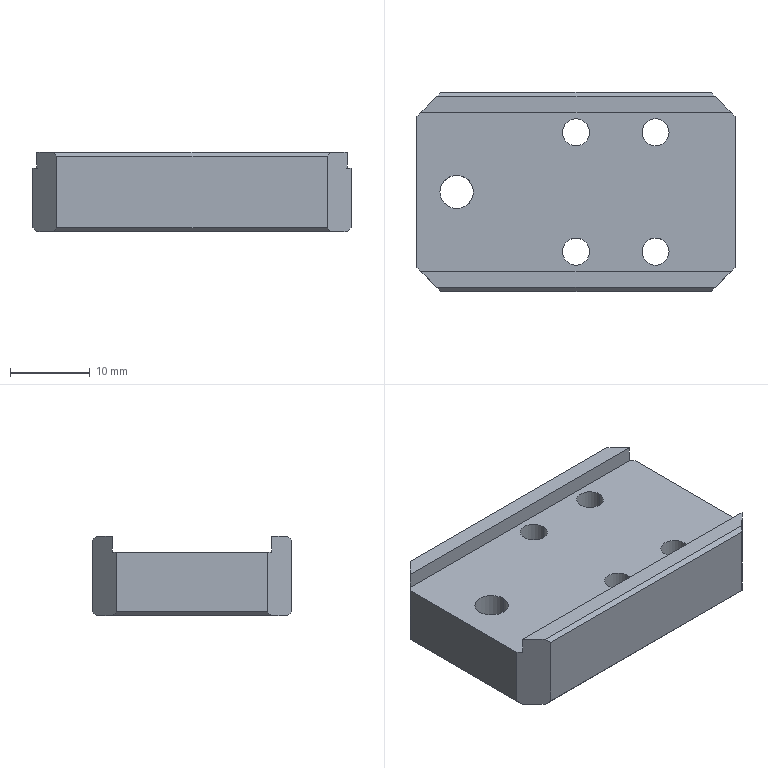Part | SolidWorks | features Chamfer 2, HoleWzd 2, Extrusion 1, ICE 1 | 1 solid | 42 faces | box 40 x 25 x 10 mm | volume 7537 mm3 | plane 24 | cylinder 18 | commonest cylinder face diameters 3.4 x8 6 x8 4.2 x2
STEP:
#1=CARTESIAN_POINT('',(13.,7.5,3.4));
#2=VERTEX_POINT('',#1);
#3=CARTESIAN_POINT('',(7.,7.5,3.4));
#4=VERTEX_POINT('',#3);
#5=CARTESIAN_POINT('',(10.,7.5,3.4));
#6=DIRECTION('',(0.,0.,-1.));
#7=DIRECTION('',(-1.,0.,0.));
#8=AXIS2_PLACEMENT_3D('',#5,#6,#7);
#9=CIRCLE('',#8,3.);
#10=EDGE_CURVE('',#2,#4,#9,.T.);
#11=ORIENTED_EDGE('',*,*,#10,.F.);
#12=CARTESIAN_POINT('',(13.,7.5,0.));
#13=VERTEX_POINT('',#12);
#14=CARTESIAN_POINT('',(13.,7.5,0.));
#15=DIRECTION('',(0.,0.,-1.));
#16=VECTOR('',#15,1000.);
#17=LINE('',#14,#16);
#18=EDGE_CURVE('',#2,#13,#17,.T.);
#19=ORIENTED_EDGE('',*,*,#18,.T.);
#20=CARTESIAN_POINT('',(7.,7.5,0.));
#21=VERTEX_POINT('',#20);
#22=CARTESIAN_POINT('',(10.,7.5,0.));
#23=DIRECTION('',(0.,0.,-1.));
#24=DIRECTION('',(-1.,0.,0.));
#25=AXIS2_PLACEMENT_3D('',#22,#23,#24);
#26=CIRCLE('',#25,3.);
#27=EDGE_CURVE('',#13,#21,#26,.T.);
#28=ORIENTED_EDGE('',*,*,#27,.T.);
#29=CARTESIAN_POINT('',(7.,7.5,0.));
#30=DIRECTION('',(0.,0.,-1.));
#31=VECTOR('',#30,1000.);
#32=LINE('',#29,#31);
#33=EDGE_CURVE('',#4,#21,#32,.T.);
#34=ORIENTED_EDGE('',*,*,#33,.F.);
#35=EDGE_LOOP('',(#11,#19,#28,#34));
#36=FACE_OUTER_BOUND('',#35,.T.);
#37=CARTESIAN_POINT('',(10.,7.5,0.));
#38=DIRECTION('',(0.,0.,-1.));
#39=DIRECTION('',(-1.,0.,0.));
#40=AXIS2_PLACEMENT_3D('',#37,#38,#39);
#41=CYLINDRICAL_SURFACE('',#40,3.);
#42=ADVANCED_FACE('',(#36),#41,.F.);
#43=CARTESIAN_POINT('',(11.7,7.5,8.));
#44=VERTEX_POINT('',#43);
#45=CARTESIAN_POINT('',(8.3,7.5,8.));
#46=VERTEX_POINT('',#45);
#47=CARTESIAN_POINT('',(10.,7.5,8.));
#48=DIRECTION('',(0.,0.,-1.));
#49=DIRECTION('',(-1.,0.,0.));
#50=AXIS2_PLACEMENT_3D('',#47,#48,#49);
#51=CIRCLE('',#50,1.7);
#52=EDGE_CURVE('',#44,#46,#51,.T.);
#53=ORIENTED_EDGE('',*,*,#52,.F.);
#54=CARTESIAN_POINT('',(11.7,7.5,3.4));
#55=VERTEX_POINT('',#54);
#56=CARTESIAN_POINT('',(11.7,7.5,0.));
#57=DIRECTION('',(0.,0.,-1.));
#58=VECTOR('',#57,1000.);
#59=LINE('',#56,#58);
#60=EDGE_CURVE('',#44,#55,#59,.T.);
#61=ORIENTED_EDGE('',*,*,#60,.T.);
#62=CARTESIAN_POINT('',(8.3,7.5,3.4));
#63=VERTEX_POINT('',#62);
#64=CARTESIAN_POINT('',(10.,7.5,3.4));
#65=DIRECTION('',(0.,0.,-1.));
#66=DIRECTION('',(-1.,0.,0.));
#67=AXIS2_PLACEMENT_3D('',#64,#65,#66);
#68=CIRCLE('',#67,1.7);
#69=EDGE_CURVE('',#55,#63,#68,.T.);
#70=ORIENTED_EDGE('',*,*,#69,.T.);
#71=CARTESIAN_POINT('',(8.3,7.5,0.));
#72=DIRECTION('',(0.,0.,-1.));
#73=VECTOR('',#72,1000.);
#74=LINE('',#71,#73);
#75=EDGE_CURVE('',#46,#63,#74,.T.);
#76=ORIENTED_EDGE('',*,*,#75,.F.);
#77=EDGE_LOOP('',(#53,#61,#70,#76));
#78=FACE_OUTER_BOUND('',#77,.T.);
#79=CARTESIAN_POINT('',(10.,7.5,0.));
#80=DIRECTION('',(0.,0.,-1.));
#81=DIRECTION('',(-1.,0.,0.));
#82=AXIS2_PLACEMENT_3D('',#79,#80,#81);
#83=CYLINDRICAL_SURFACE('',#82,1.7);
#84=ADVANCED_FACE('',(#78),#83,.F.);
#85=CARTESIAN_POINT('',(13.,-7.5,3.4));
#86=VERTEX_POINT('',#85);
#87=CARTESIAN_POINT('',(7.,-7.5,3.4));
#88=VERTEX_POINT('',#87);
#89=CARTESIAN_POINT('',(10.,-7.5,3.4));
#90=DIRECTION('',(0.,0.,-1.));
#91=DIRECTION('',(-1.,0.,0.));
#92=AXIS2_PLACEMENT_3D('',#89,#90,#91);
#93=CIRCLE('',#92,3.);
#94=EDGE_CURVE('',#86,#88,#93,.T.);
#95=ORIENTED_EDGE('',*,*,#94,.F.);
#96=CARTESIAN_POINT('',(13.,-7.5,0.));
#97=VERTEX_POINT('',#96);
#98=CARTESIAN_POINT('',(13.,-7.5,0.));
#99=DIRECTION('',(0.,0.,-1.));
#100=VECTOR('',#99,1000.);
#101=LINE('',#98,#100);
#102=EDGE_CURVE('',#86,#97,#101,.T.);
#103=ORIENTED_EDGE('',*,*,#102,.T.);
#104=CARTESIAN_POINT('',(7.,-7.5,0.));
#105=VERTEX_POINT('',#104);
#106=CARTESIAN_POINT('',(10.,-7.5,0.));
#107=DIRECTION('',(0.,0.,-1.));
#108=DIRECTION('',(-1.,0.,0.));
#109=AXIS2_PLACEMENT_3D('',#106,#107,#108);
#110=CIRCLE('',#109,3.);
#111=EDGE_CURVE('',#97,#105,#110,.T.);
#112=ORIENTED_EDGE('',*,*,#111,.T.);
#113=CARTESIAN_POINT('',(7.,-7.5,0.));
#114=DIRECTION('',(0.,0.,-1.));
#115=VECTOR('',#114,1000.);
#116=LINE('',#113,#115);
#117=EDGE_CURVE('',#88,#105,#116,.T.);
#118=ORIENTED_EDGE('',*,*,#117,.F.);
#119=EDGE_LOOP('',(#95,#103,#112,#118));
#120=FACE_OUTER_BOUND('',#119,.T.);
#121=CARTESIAN_POINT('',(10.,-7.5,0.));
#122=DIRECTION('',(0.,0.,-1.));
#123=DIRECTION('',(-1.,0.,0.));
#124=AXIS2_PLACEMENT_3D('',#121,#122,#123);
#125=CYLINDRICAL_SURFACE('',#124,3.);
#126=ADVANCED_FACE('',(#120),#125,.F.);
#127=CARTESIAN_POINT('',(11.7,-7.5,8.));
#128=VERTEX_POINT('',#127);
#129=CARTESIAN_POINT('',(8.3,-7.5,8.));
#130=VERTEX_POINT('',#129);
#131=CARTESIAN_POINT('',(10.,-7.5,8.));
#132=DIRECTION('',(0.,0.,-1.));
#133=DIRECTION('',(-1.,0.,0.));
#134=AXIS2_PLACEMENT_3D('',#131,#132,#133);
#135=CIRCLE('',#134,1.7);
#136=EDGE_CURVE('',#128,#130,#135,.T.);
#137=ORIENTED_EDGE('',*,*,#136,.F.);
#138=CARTESIAN_POINT('',(11.7,-7.5,3.4));
#139=VERTEX_POINT('',#138);
#140=CARTESIAN_POINT('',(11.7,-7.5,0.));
#141=DIRECTION('',(0.,0.,-1.));
#142=VECTOR('',#141,1000.);
#143=LINE('',#140,#142);
#144=EDGE_CURVE('',#128,#139,#143,.T.);
#145=ORIENTED_EDGE('',*,*,#144,.T.);
#146=CARTESIAN_POINT('',(8.3,-7.5,3.4));
#147=VERTEX_POINT('',#146);
#148=CARTESIAN_POINT('',(10.,-7.5,3.4));
#149=DIRECTION('',(0.,0.,-1.));
#150=DIRECTION('',(-1.,0.,0.));
#151=AXIS2_PLACEMENT_3D('',#148,#149,#150);
#152=CIRCLE('',#151,1.7);
#153=EDGE_CURVE('',#139,#147,#152,.T.);
#154=ORIENTED_EDGE('',*,*,#153,.T.);
#155=CARTESIAN_POINT('',(8.3,-7.5,0.));
#156=DIRECTION('',(0.,0.,-1.));
#157=VECTOR('',#156,1000.);
#158=LINE('',#155,#157);
#159=EDGE_CURVE('',#130,#147,#158,.T.);
#160=ORIENTED_EDGE('',*,*,#159,.F.);
#161=EDGE_LOOP('',(#137,#145,#154,#160));
#162=FACE_OUTER_BOUND('',#161,.T.);
#163=CARTESIAN_POINT('',(10.,-7.5,0.));
#164=DIRECTION('',(0.,0.,-1.));
#165=DIRECTION('',(-1.,0.,0.));
#166=AXIS2_PLACEMENT_3D('',#163,#164,#165);
#167=CYLINDRICAL_SURFACE('',#166,1.7);
#168=ADVANCED_FACE('',(#162),#167,.F.);
#169=CARTESIAN_POINT('',(3.,7.5,3.4));
#170=VERTEX_POINT('',#169);
#171=CARTESIAN_POINT('',(-3.,7.5,3.4));
#172=VERTEX_POINT('',#171);
#173=CARTESIAN_POINT('',(0.,7.5,3.4));
#174=DIRECTION('',(0.,0.,-1.));
#175=DIRECTION('',(-1.,0.,0.));
#176=AXIS2_PLACEMENT_3D('',#173,#174,#175);
#177=CIRCLE('',#176,3.);
#178=EDGE_CURVE('',#170,#172,#177,.T.);
#179=ORIENTED_EDGE('',*,*,#178,.F.);
#180=CARTESIAN_POINT('',(3.,7.5,0.));
#181=VERTEX_POINT('',#180);
#182=CARTESIAN_POINT('',(3.,7.5,0.));
#183=DIRECTION('',(0.,0.,-1.));
#184=VECTOR('',#183,1000.);
#185=LINE('',#182,#184);
#186=EDGE_CURVE('',#170,#181,#185,.T.);
#187=ORIENTED_EDGE('',*,*,#186,.T.);
#188=CARTESIAN_POINT('',(-3.,7.5,0.));
#189=VERTEX_POINT('',#188);
#190=CARTESIAN_POINT('',(0.,7.5,0.));
#191=DIRECTION('',(0.,0.,-1.));
#192=DIRECTION('',(-1.,0.,0.));
#193=AXIS2_PLACEMENT_3D('',#190,#191,#192);
#194=CIRCLE('',#193,3.);
#195=EDGE_CURVE('',#181,#189,#194,.T.);
#196=ORIENTED_EDGE('',*,*,#195,.T.);
#197=CARTESIAN_POINT('',(-3.,7.5,0.));
#198=DIRECTION('',(0.,0.,-1.));
#199=VECTOR('',#198,1000.);
#200=LINE('',#197,#199);
#201=EDGE_CURVE('',#172,#189,#200,.T.);
#202=ORIENTED_EDGE('',*,*,#201,.F.);
#203=EDGE_LOOP('',(#179,#187,#196,#202));
#204=FACE_OUTER_BOUND('',#203,.T.);
#205=CARTESIAN_POINT('',(0.,7.5,0.));
#206=DIRECTION('',(0.,0.,-1.));
#207=DIRECTION('',(-1.,0.,0.));
#208=AXIS2_PLACEMENT_3D('',#205,#206,#207);
#209=CYLINDRICAL_SURFACE('',#208,3.);
#210=ADVANCED_FACE('',(#204),#209,.F.);
#211=CARTESIAN_POINT('',(1.7,7.5,8.));
#212=VERTEX_POINT('',#211);
#213=CARTESIAN_POINT('',(-1.7,7.5,8.));
#214=VERTEX_POINT('',#213);
#215=CARTESIAN_POINT('',(0.,7.5,8.));
#216=DIRECTION('',(0.,0.,-1.));
#217=DIRECTION('',(-1.,0.,0.));
#218=AXIS2_PLACEMENT_3D('',#215,#216,#217);
#219=CIRCLE('',#218,1.7);
#220=EDGE_CURVE('',#212,#214,#219,.T.);
#221=ORIENTED_EDGE('',*,*,#220,.F.);
#222=CARTESIAN_POINT('',(1.7,7.5,3.4));
#223=VERTEX_POINT('',#222);
#224=CARTESIAN_POINT('',(1.7,7.5,0.));
#225=DIRECTION('',(0.,0.,-1.));
#226=VECTOR('',#225,1000.);
#227=LINE('',#224,#226);
#228=EDGE_CURVE('',#212,#223,#227,.T.);
#229=ORIENTED_EDGE('',*,*,#228,.T.);
#230=CARTESIAN_POINT('',(-1.7,7.5,3.4));
#231=VERTEX_POINT('',#230);
#232=CARTESIAN_POINT('',(0.,7.5,3.4));
#233=DIRECTION('',(0.,0.,-1.));
#234=DIRECTION('',(-1.,0.,0.));
#235=AXIS2_PLACEMENT_3D('',#232,#233,#234);
#236=CIRCLE('',#235,1.7);
#237=EDGE_CURVE('',#223,#231,#236,.T.);
#238=ORIENTED_EDGE('',*,*,#237,.T.);
#239=CARTESIAN_POINT('',(-1.7,7.5,0.));
#240=DIRECTION('',(0.,0.,-1.));
#241=VECTOR('',#240,1000.);
#242=LINE('',#239,#241);
#243=EDGE_CURVE('',#214,#231,#242,.T.);
#244=ORIENTED_EDGE('',*,*,#243,.F.);
#245=EDGE_LOOP('',(#221,#229,#238,#244));
#246=FACE_OUTER_BOUND('',#245,.T.);
#247=CARTESIAN_POINT('',(0.,7.5,0.));
#248=DIRECTION('',(0.,0.,-1.));
#249=DIRECTION('',(-1.,0.,0.));
#250=AXIS2_PLACEMENT_3D('',#247,#248,#249);
#251=CYLINDRICAL_SURFACE('',#250,1.7);
#252=ADVANCED_FACE('',(#246),#251,.F.);
#253=CARTESIAN_POINT('',(3.,-7.5,3.4));
#254=VERTEX_POINT('',#253);
#255=CARTESIAN_POINT('',(-3.,-7.5,3.4));
#256=VERTEX_POINT('',#255);
#257=CARTESIAN_POINT('',(0.,-7.5,3.4));
#258=DIRECTION('',(0.,0.,-1.));
#259=DIRECTION('',(-1.,0.,0.));
#260=AXIS2_PLACEMENT_3D('',#257,#258,#259);
#261=CIRCLE('',#260,3.);
#262=EDGE_CURVE('',#254,#256,#261,.T.);
#263=ORIENTED_EDGE('',*,*,#262,.F.);
#264=CARTESIAN_POINT('',(3.,-7.5,0.));
#265=VERTEX_POINT('',#264);
#266=CARTESIAN_POINT('',(3.,-7.5,0.));
#267=DIRECTION('',(0.,0.,-1.));
#268=VECTOR('',#267,1000.);
#269=LINE('',#266,#268);
#270=EDGE_CURVE('',#254,#265,#269,.T.);
#271=ORIENTED_EDGE('',*,*,#270,.T.);
#272=CARTESIAN_POINT('',(-3.,-7.5,0.));
#273=VERTEX_POINT('',#272);
#274=CARTESIAN_POINT('',(0.,-7.5,0.));
#275=DIRECTION('',(0.,0.,-1.));
#276=DIRECTION('',(-1.,0.,0.));
#277=AXIS2_PLACEMENT_3D('',#274,#275,#276);
#278=CIRCLE('',#277,3.);
#279=EDGE_CURVE('',#265,#273,#278,.T.);
#280=ORIENTED_EDGE('',*,*,#279,.T.);
#281=CARTESIAN_POINT('',(-3.,-7.5,0.));
#282=DIRECTION('',(0.,0.,-1.));
#283=VECTOR('',#282,1000.);
#284=LINE('',#281,#283);
#285=EDGE_CURVE('',#256,#273,#284,.T.);
#286=ORIENTED_EDGE('',*,*,#285,.F.);
#287=EDGE_LOOP('',(#263,#271,#280,#286));
#288=FACE_OUTER_BOUND('',#287,.T.);
#289=CARTESIAN_POINT('',(0.,-7.5,0.));
#290=DIRECTION('',(0.,0.,-1.));
#291=DIRECTION('',(-1.,0.,0.));
#292=AXIS2_PLACEMENT_3D('',#289,#290,#291);
#293=CYLINDRICAL_SURFACE('',#292,3.);
#294=ADVANCED_FACE('',(#288),#293,.F.);
#295=CARTESIAN_POINT('',(1.7,-7.5,8.));
#296=VERTEX_POINT('',#295);
#297=CARTESIAN_POINT('',(-1.7,-7.5,8.));
#298=VERTEX_POINT('',#297);
#299=CARTESIAN_POINT('',(0.,-7.5,8.));
#300=DIRECTION('',(0.,0.,-1.));
#301=DIRECTION('',(-1.,0.,0.));
#302=AXIS2_PLACEMENT_3D('',#299,#300,#301);
#303=CIRCLE('',#302,1.7);
#304=EDGE_CURVE('',#296,#298,#303,.T.);
#305=ORIENTED_EDGE('',*,*,#304,.F.);
#306=CARTESIAN_POINT('',(1.7,-7.5,3.4));
#307=VERTEX_POINT('',#306);
#308=CARTESIAN_POINT('',(1.7,-7.5,0.));
#309=DIRECTION('',(0.,0.,-1.));
#310=VECTOR('',#309,1000.);
#311=LINE('',#308,#310);
#312=EDGE_CURVE('',#296,#307,#311,.T.);
#313=ORIENTED_EDGE('',*,*,#312,.T.);
#314=CARTESIAN_POINT('',(-1.7,-7.5,3.4));
#315=VERTEX_POINT('',#314);
#316=CARTESIAN_POINT('',(0.,-7.5,3.4));
#317=DIRECTION('',(0.,0.,-1.));
#318=DIRECTION('',(-1.,0.,0.));
#319=AXIS2_PLACEMENT_3D('',#316,#317,#318);
#320=CIRCLE('',#319,1.7);
#321=EDGE_CURVE('',#307,#315,#320,.T.);
#322=ORIENTED_EDGE('',*,*,#321,.T.);
#323=CARTESIAN_POINT('',(-1.7,-7.5,0.));
#324=DIRECTION('',(0.,0.,-1.));
#325=VECTOR('',#324,1000.);
#326=LINE('',#323,#325);
#327=EDGE_CURVE('',#298,#315,#326,.T.);
#328=ORIENTED_EDGE('',*,*,#327,.F.);
#329=EDGE_LOOP('',(#305,#313,#322,#328));
#330=FACE_OUTER_BOUND('',#329,.T.);
#331=CARTESIAN_POINT('',(0.,-7.5,0.));
#332=DIRECTION('',(0.,0.,-1.));
#333=DIRECTION('',(-1.,0.,0.));
#334=AXIS2_PLACEMENT_3D('',#331,#332,#333);
#335=CYLINDRICAL_SURFACE('',#334,1.7);
#336=ADVANCED_FACE('',(#330),#335,.F.);
#337=CARTESIAN_POINT('',(-17.1,0.,0.));
#338=VERTEX_POINT('',#337);
#339=CARTESIAN_POINT('',(-12.9,0.,0.));
#340=VERTEX_POINT('',#339);
#341=CARTESIAN_POINT('',(-15.,0.,0.));
#342=DIRECTION('',(0.,0.,1.));
#343=DIRECTION('',(1.,0.,0.));
#344=AXIS2_PLACEMENT_3D('',#341,#342,#343);
#345=CIRCLE('',#344,2.1);
#346=EDGE_CURVE('',#338,#340,#345,.T.);
#347=ORIENTED_EDGE('',*,*,#346,.F.);
#348=CARTESIAN_POINT('',(-17.1,0.,8.));
#349=VERTEX_POINT('',#348);
#350=CARTESIAN_POINT('',(-17.1,0.,8.));
#351=DIRECTION('',(0.,0.,1.));
#352=VECTOR('',#351,1000.);
#353=LINE('',#350,#352);
#354=EDGE_CURVE('',#338,#349,#353,.T.);
#355=ORIENTED_EDGE('',*,*,#354,.T.);
#356=CARTESIAN_POINT('',(-12.9,0.,8.));
#357=VERTEX_POINT('',#356);
#358=CARTESIAN_POINT('',(-15.,0.,8.));
#359=DIRECTION('',(0.,0.,1.));
#360=DIRECTION('',(1.,0.,0.));
#361=AXIS2_PLACEMENT_3D('',#358,#359,#360);
#362=CIRCLE('',#361,2.1);
#363=EDGE_CURVE('',#349,#357,#362,.T.);
#364=ORIENTED_EDGE('',*,*,#363,.T.);
#365=CARTESIAN_POINT('',(-12.9,0.,8.));
#366=DIRECTION('',(0.,0.,1.));
#367=VECTOR('',#366,1000.);
#368=LINE('',#365,#367);
#369=EDGE_CURVE('',#340,#357,#368,.T.);
#370=ORIENTED_EDGE('',*,*,#369,.F.);
#371=EDGE_LOOP('',(#347,#355,#364,#370));
#372=FACE_OUTER_BOUND('',#371,.T.);
#373=CARTESIAN_POINT('',(-15.,0.,8.));
#374=DIRECTION('',(0.,0.,1.));
#375=DIRECTION('',(1.,0.,0.));
#376=AXIS2_PLACEMENT_3D('',#373,#374,#375);
#377=CYLINDRICAL_SURFACE('',#376,2.1);
#378=ADVANCED_FACE('',(#372),#377,.F.);
#379=CARTESIAN_POINT('',(-19.5,-10.,10.));
#380=VERTEX_POINT('',#379);
#381=CARTESIAN_POINT('',(-17.5,-12.,10.));
#382=VERTEX_POINT('',#381);
#383=CARTESIAN_POINT('',(-17.,-12.5,10.));
#384=DIRECTION('',(0.7071,-0.7071,0.));
#385=VECTOR('',#384,1000.);
#386=LINE('',#383,#385);
#387=EDGE_CURVE('',#380,#382,#386,.T.);
#388=ORIENTED_EDGE('',*,*,#387,.T.);
#389=CARTESIAN_POINT('',(17.5,-12.,10.));
#390=VERTEX_POINT('',#389);
#391=CARTESIAN_POINT('',(0.,-12.,10.));
#392=DIRECTION('',(1.,0.,0.));
#393=VECTOR('',#392,1000.);
#394=LINE('',#391,#393);
#395=EDGE_CURVE('',#382,#390,#394,.T.);
#396=ORIENTED_EDGE('',*,*,#395,.T.);
#397=CARTESIAN_POINT('',(19.5,-10.,10.));
#398=VERTEX_POINT('',#397);
#399=CARTESIAN_POINT('',(20.,-9.5,10.));
#400=DIRECTION('',(0.7071,0.7071,0.));
#401=VECTOR('',#400,1000.);
#402=LINE('',#399,#401);
#403=EDGE_CURVE('',#390,#398,#402,.T.);
#404=ORIENTED_EDGE('',*,*,#403,.T.);
#405=CARTESIAN_POINT('',(-20.,-10.,10.));
#406=DIRECTION('',(1.,0.,0.));
#407=VECTOR('',#406,1000.);
#408=LINE('',#405,#407);
#409=EDGE_CURVE('',#380,#398,#408,.T.);
#410=ORIENTED_EDGE('',*,*,#409,.F.);
#411=EDGE_LOOP('',(#388,#396,#404,#410));
#412=FACE_OUTER_BOUND('',#411,.T.);
#413=CARTESIAN_POINT('',(0.,0.,10.));
#414=DIRECTION('',(0.,0.,-1.));
#415=DIRECTION('',(-1.,0.,0.));
#416=AXIS2_PLACEMENT_3D('',#413,#414,#415);
#417=PLANE('',#416);
#418=ADVANCED_FACE('',(#412),#417,.F.);
#419=CARTESIAN_POINT('',(20.,-9.5,8.));
#420=VERTEX_POINT('',#419);
#421=CARTESIAN_POINT('',(20.,-9.5,0.5));
#422=VERTEX_POINT('',#421);
#423=CARTESIAN_POINT('',(20.,-9.5,10.));
#424=DIRECTION('',(0.,0.,-1.));
#425=VECTOR('',#424,1000.);
#426=LINE('',#423,#425);
#427=EDGE_CURVE('',#420,#422,#426,.T.);
#428=ORIENTED_EDGE('',*,*,#427,.T.);
#429=CARTESIAN_POINT('',(20.,9.5,0.5));
#430=VERTEX_POINT('',#429);
#431=CARTESIAN_POINT('',(20.,9.5,0.5));
#432=DIRECTION('',(0.,1.,0.));
#433=VECTOR('',#432,1000.);
#434=LINE('',#431,#433);
#435=EDGE_CURVE('',#422,#430,#434,.T.);
#436=ORIENTED_EDGE('',*,*,#435,.T.);
#437=CARTESIAN_POINT('',(20.,9.5,8.));
#438=VERTEX_POINT('',#437);
#439=CARTESIAN_POINT('',(20.,9.5,10.));
#440=DIRECTION('',(0.,0.,1.));
#441=VECTOR('',#440,1000.);
#442=LINE('',#439,#441);
#443=EDGE_CURVE('',#430,#438,#442,.T.);
#444=ORIENTED_EDGE('',*,*,#443,.T.);
#445=CARTESIAN_POINT('',(20.,-10.,8.));
#446=DIRECTION('',(0.,1.,0.));
#447=VECTOR('',#446,1000.);
#448=LINE('',#445,#447);
#449=EDGE_CURVE('',#420,#438,#448,.T.);
#450=ORIENTED_EDGE('',*,*,#449,.F.);
#451=EDGE_LOOP('',(#428,#436,#444,#450));
#452=FACE_OUTER_BOUND('',#451,.T.);
#453=CARTESIAN_POINT('',(20.,-12.5,10.));
#454=DIRECTION('',(-1.,0.,0.));
#455=DIRECTION('',(0.,0.,1.));
#456=AXIS2_PLACEMENT_3D('',#453,#454,#455);
#457=PLANE('',#456);
#458=ADVANCED_FACE('',(#452),#457,.F.);
#459=CARTESIAN_POINT('',(-17.,12.5,0.5));
#460=VERTEX_POINT('',#459);
#461=CARTESIAN_POINT('',(-17.,12.5,9.5));
#462=VERTEX_POINT('',#461);
#463=CARTESIAN_POINT('',(-17.,12.5,10.));
#464=DIRECTION('',(0.,0.,1.));
#465=VECTOR('',#464,1000.);
#466=LINE('',#463,#465);
#467=EDGE_CURVE('',#460,#462,#466,.T.);
#468=ORIENTED_EDGE('',*,*,#467,.T.);
#469=CARTESIAN_POINT('',(17.,12.5,9.5));
#470=VERTEX_POINT('',#469);
#471=CARTESIAN_POINT('',(-20.,12.5,9.5));
#472=DIRECTION('',(1.,0.,0.));
#473=VECTOR('',#472,1000.);
#474=LINE('',#471,#473);
#475=EDGE_CURVE('',#462,#470,#474,.T.);
#476=ORIENTED_EDGE('',*,*,#475,.T.);
#477=CARTESIAN_POINT('',(17.,12.5,0.5));
#478=VERTEX_POINT('',#477);
#479=CARTESIAN_POINT('',(17.,12.5,10.));
#480=DIRECTION('',(0.,0.,-1.));
#481=VECTOR('',#480,1000.);
#482=LINE('',#479,#481);
#483=EDGE_CURVE('',#470,#478,#482,.T.);
#484=ORIENTED_EDGE('',*,*,#483,.T.);
#485=CARTESIAN_POINT('',(-17.,12.5,0.5));
#486=DIRECTION('',(-1.,0.,0.));
#487=VECTOR('',#486,1000.);
#488=LINE('',#485,#487);
#489=EDGE_CURVE('',#478,#460,#488,.T.);
#490=ORIENTED_EDGE('',*,*,#489,.T.);
#491=EDGE_LOOP('',(#468,#476,#484,#490));
#492=FACE_OUTER_BOUND('',#491,.T.);
#493=CARTESIAN_POINT('',(-20.,12.5,10.));
#494=DIRECTION('',(0.,-1.,0.));
#495=DIRECTION('',(0.,0.,-1.));
#496=AXIS2_PLACEMENT_3D('',#493,#494,#495);
#497=PLANE('',#496);
#498=ADVANCED_FACE('',(#492),#497,.F.);
#499=CARTESIAN_POINT('',(-20.,9.5,8.));
#500=VERTEX_POINT('',#499);
#501=CARTESIAN_POINT('',(-20.,9.5,0.5));
#502=VERTEX_POINT('',#501);
#503=CARTESIAN_POINT('',(-20.,9.5,10.));
#504=DIRECTION('',(0.,0.,-1.));
#505=VECTOR('',#504,1000.);
#506=LINE('',#503,#505);
#507=EDGE_CURVE('',#500,#502,#506,.T.);
#508=ORIENTED_EDGE('',*,*,#507,.T.);
#509=CARTESIAN_POINT('',(-20.,-9.5,0.5));
#510=VERTEX_POINT('',#509);
#511=CARTESIAN_POINT('',(-20.,-9.5,0.5));
#512=DIRECTION('',(0.,-1.,0.));
#513=VECTOR('',#512,1000.);
#514=LINE('',#511,#513);
#515=EDGE_CURVE('',#502,#510,#514,.T.);
#516=ORIENTED_EDGE('',*,*,#515,.T.);
#517=CARTESIAN_POINT('',(-20.,-9.5,8.));
#518=VERTEX_POINT('',#517);
#519=CARTESIAN_POINT('',(-20.,-9.5,10.));
#520=DIRECTION('',(0.,0.,1.));
#521=VECTOR('',#520,1000.);
#522=LINE('',#519,#521);
#523=EDGE_CURVE('',#510,#518,#522,.T.);
#524=ORIENTED_EDGE('',*,*,#523,.T.);
#525=CARTESIAN_POINT('',(-20.,-10.,8.));
#526=DIRECTION('',(0.,-1.,0.));
#527=VECTOR('',#526,1000.);
#528=LINE('',#525,#527);
#529=EDGE_CURVE('',#500,#518,#528,.T.);
#530=ORIENTED_EDGE('',*,*,#529,.F.);
#531=EDGE_LOOP('',(#508,#516,#524,#530));
#532=FACE_OUTER_BOUND('',#531,.T.);
#533=CARTESIAN_POINT('',(-20.,-12.5,10.));
#534=DIRECTION('',(1.,0.,0.));
#535=DIRECTION('',(0.,0.,-1.));
#536=AXIS2_PLACEMENT_3D('',#533,#534,#535);
#537=PLANE('',#536);
#538=ADVANCED_FACE('',(#532),#537,.F.);
#539=CARTESIAN_POINT('',(17.,-12.5,0.5));
#540=VERTEX_POINT('',#539);
#541=CARTESIAN_POINT('',(17.,-12.5,9.5));
#542=VERTEX_POINT('',#541);
#543=CARTESIAN_POINT('',(17.,-12.5,10.));
#544=DIRECTION('',(0.,0.,1.));
#545=VECTOR('',#544,1000.);
#546=LINE('',#543,#545);
#547=EDGE_CURVE('',#540,#542,#546,.T.);
#548=ORIENTED_EDGE('',*,*,#547,.T.);
#549=CARTESIAN_POINT('',(-17.,-12.5,9.5));
#550=VERTEX_POINT('',#549);
#551=CARTESIAN_POINT('',(-20.,-12.5,9.5));
#552=DIRECTION('',(-1.,0.,0.));
#553=VECTOR('',#552,1000.);
#554=LINE('',#551,#553);
#555=EDGE_CURVE('',#542,#550,#554,.T.);
#556=ORIENTED_EDGE('',*,*,#555,.T.);
#557=CARTESIAN_POINT('',(-17.,-12.5,0.5));
#558=VERTEX_POINT('',#557);
#559=CARTESIAN_POINT('',(-17.,-12.5,10.));
#560=DIRECTION('',(0.,0.,-1.));
#561=VECTOR('',#560,1000.);
#562=LINE('',#559,#561);
#563=EDGE_CURVE('',#550,#558,#562,.T.);
#564=ORIENTED_EDGE('',*,*,#563,.T.);
#565=CARTESIAN_POINT('',(17.,-12.5,0.5));
#566=DIRECTION('',(1.,0.,0.));
#567=VECTOR('',#566,1000.);
#568=LINE('',#565,#567);
#569=EDGE_CURVE('',#558,#540,#568,.T.);
#570=ORIENTED_EDGE('',*,*,#569,.T.);
#571=EDGE_LOOP('',(#548,#556,#564,#570));
#572=FACE_OUTER_BOUND('',#571,.T.);
#573=CARTESIAN_POINT('',(-20.,-12.5,10.));
#574=DIRECTION('',(0.,1.,0.));
#575=DIRECTION('',(0.,0.,1.));
#576=AXIS2_PLACEMENT_3D('',#573,#574,#575);
#577=PLANE('',#576);
#578=ADVANCED_FACE('',(#572),#577,.F.);
#579=CARTESIAN_POINT('',(19.5,10.,10.));
#580=VERTEX_POINT('',#579);
#581=CARTESIAN_POINT('',(17.5,12.,10.));
#582=VERTEX_POINT('',#581);
#583=CARTESIAN_POINT('',(17.,12.5,10.));
#584=DIRECTION('',(-0.7071,0.7071,0.));
#585=VECTOR('',#584,1000.);
#586=LINE('',#583,#585);
#587=EDGE_CURVE('',#580,#582,#586,.T.);
#588=ORIENTED_EDGE('',*,*,#587,.T.);
#589=CARTESIAN_POINT('',(-17.5,12.,10.));
#590=VERTEX_POINT('',#589);
#591=CARTESIAN_POINT('',(0.,12.,10.));
#592=DIRECTION('',(-1.,0.,0.));
#593=VECTOR('',#592,1000.);
#594=LINE('',#591,#593);
#595=EDGE_CURVE('',#582,#590,#594,.T.);
#596=ORIENTED_EDGE('',*,*,#595,.T.);
#597=CARTESIAN_POINT('',(-19.5,10.,10.));
#598=VERTEX_POINT('',#597);
#599=CARTESIAN_POINT('',(-20.,9.5,10.));
#600=DIRECTION('',(-0.7071,-0.7071,0.));
#601=VECTOR('',#600,1000.);
#602=LINE('',#599,#601);
#603=EDGE_CURVE('',#590,#598,#602,.T.);
#604=ORIENTED_EDGE('',*,*,#603,.T.);
#605=CARTESIAN_POINT('',(-20.,10.,10.));
#606=DIRECTION('',(-1.,0.,0.));
#607=VECTOR('',#606,1000.);
#608=LINE('',#605,#607);
#609=EDGE_CURVE('',#580,#598,#608,.T.);
#610=ORIENTED_EDGE('',*,*,#609,.F.);
#611=EDGE_LOOP('',(#588,#596,#604,#610));
#612=FACE_OUTER_BOUND('',#611,.T.);
#613=CARTESIAN_POINT('',(0.,0.,10.));
#614=DIRECTION('',(0.,0.,-1.));
#615=DIRECTION('',(-1.,0.,0.));
#616=AXIS2_PLACEMENT_3D('',#613,#614,#615);
#617=PLANE('',#616);
#618=ADVANCED_FACE('',(#612),#617,.F.);
#619=CARTESIAN_POINT('',(10.,7.5,0.));
#620=DIRECTION('',(0.,0.,-1.));
#621=DIRECTION('',(-1.,0.,0.));
#622=AXIS2_PLACEMENT_3D('',#619,#620,#621);
#623=CIRCLE('',#622,3.);
#624=EDGE_CURVE('',#21,#13,#623,.T.);
#625=ORIENTED_EDGE('',*,*,#624,.F.);
#626=ORIENTED_EDGE('',*,*,#27,.F.);
#627=EDGE_LOOP('',(#625,#626));
#628=FACE_BOUND('',#627,.T.);
#629=CARTESIAN_POINT('',(10.,-7.5,0.));
#630=DIRECTION('',(0.,0.,-1.));
#631=DIRECTION('',(-1.,0.,0.));
#632=AXIS2_PLACEMENT_3D('',#629,#630,#631);
#633=CIRCLE('',#632,3.);
#634=EDGE_CURVE('',#105,#97,#633,.T.);
#635=ORIENTED_EDGE('',*,*,#634,.F.);
#636=ORIENTED_EDGE('',*,*,#111,.F.);
#637=EDGE_LOOP('',(#635,#636));
#638=FACE_BOUND('',#637,.T.);
#639=CARTESIAN_POINT('',(0.,7.5,0.));
#640=DIRECTION('',(0.,0.,-1.));
#641=DIRECTION('',(-1.,0.,0.));
#642=AXIS2_PLACEMENT_3D('',#639,#640,#641);
#643=CIRCLE('',#642,3.);
#644=EDGE_CURVE('',#189,#181,#643,.T.);
#645=ORIENTED_EDGE('',*,*,#644,.F.);
#646=ORIENTED_EDGE('',*,*,#195,.F.);
#647=EDGE_LOOP('',(#645,#646));
#648=FACE_BOUND('',#647,.T.);
#649=CARTESIAN_POINT('',(0.,-7.5,0.));
#650=DIRECTION('',(0.,0.,-1.));
#651=DIRECTION('',(-1.,0.,0.));
#652=AXIS2_PLACEMENT_3D('',#649,#650,#651);
#653=CIRCLE('',#652,3.);
#654=EDGE_CURVE('',#273,#265,#653,.T.);
#655=ORIENTED_EDGE('',*,*,#654,.F.);
#656=ORIENTED_EDGE('',*,*,#279,.F.);
#657=EDGE_LOOP('',(#655,#656));
#658=FACE_BOUND('',#657,.T.);
#659=CARTESIAN_POINT('',(-15.,0.,0.));
#660=DIRECTION('',(0.,0.,1.));
#661=DIRECTION('',(1.,0.,0.));
#662=AXIS2_PLACEMENT_3D('',#659,#660,#661);
#663=CIRCLE('',#662,2.1);
#664=EDGE_CURVE('',#340,#338,#663,.T.);
#665=ORIENTED_EDGE('',*,*,#664,.T.);
#666=ORIENTED_EDGE('',*,*,#346,.T.);
#667=EDGE_LOOP('',(#665,#666));
#668=FACE_BOUND('',#667,.T.);
#669=CARTESIAN_POINT('',(-17.5,-12.,0.));
#670=VERTEX_POINT('',#669);
#671=CARTESIAN_POINT('',(-19.5,-10.,0.));
#672=VERTEX_POINT('',#671);
#673=CARTESIAN_POINT('',(-14.75,-14.75,0.));
#674=DIRECTION('',(-0.7071,0.7071,0.));
#675=VECTOR('',#674,1000.);
#676=LINE('',#673,#675);
#677=EDGE_CURVE('',#670,#672,#676,.T.);
#678=ORIENTED_EDGE('',*,*,#677,.T.);
#679=CARTESIAN_POINT('',(-19.5,10.,0.));
#680=VERTEX_POINT('',#679);
#681=CARTESIAN_POINT('',(-19.5,9.5,0.));
#682=DIRECTION('',(0.,1.,0.));
#683=VECTOR('',#682,1000.);
#684=LINE('',#681,#683);
#685=EDGE_CURVE('',#672,#680,#684,.T.);
#686=ORIENTED_EDGE('',*,*,#685,.T.);
#687=CARTESIAN_POINT('',(-17.5,12.,0.));
#688=VERTEX_POINT('',#687);
#689=CARTESIAN_POINT('',(-14.75,14.75,0.));
#690=DIRECTION('',(0.7071,0.7071,0.));
#691=VECTOR('',#690,1000.);
#692=LINE('',#689,#691);
#693=EDGE_CURVE('',#680,#688,#692,.T.);
#694=ORIENTED_EDGE('',*,*,#693,.T.);
#695=CARTESIAN_POINT('',(17.5,12.,0.));
#696=VERTEX_POINT('',#695);
#697=CARTESIAN_POINT('',(17.,12.,0.));
#698=DIRECTION('',(1.,0.,0.));
#699=VECTOR('',#698,1000.);
#700=LINE('',#697,#699);
#701=EDGE_CURVE('',#688,#696,#700,.T.);
#702=ORIENTED_EDGE('',*,*,#701,.T.);
#703=CARTESIAN_POINT('',(19.5,10.,0.));
#704=VERTEX_POINT('',#703);
#705=CARTESIAN_POINT('',(14.75,14.75,0.));
#706=DIRECTION('',(0.7071,-0.7071,0.));
#707=VECTOR('',#706,1000.);
#708=LINE('',#705,#707);
#709=EDGE_CURVE('',#696,#704,#708,.T.);
#710=ORIENTED_EDGE('',*,*,#709,.T.);
#711=CARTESIAN_POINT('',(19.5,-10.,0.));
#712=VERTEX_POINT('',#711);
#713=CARTESIAN_POINT('',(19.5,-9.5,0.));
#714=DIRECTION('',(0.,-1.,0.));
#715=VECTOR('',#714,1000.);
#716=LINE('',#713,#715);
#717=EDGE_CURVE('',#704,#712,#716,.T.);
#718=ORIENTED_EDGE('',*,*,#717,.T.);
#719=CARTESIAN_POINT('',(17.5,-12.,0.));
#720=VERTEX_POINT('',#719);
#721=CARTESIAN_POINT('',(14.75,-14.75,0.));
#722=DIRECTION('',(-0.7071,-0.7071,0.));
#723=VECTOR('',#722,1000.);
#724=LINE('',#721,#723);
#725=EDGE_CURVE('',#712,#720,#724,.T.);
#726=ORIENTED_EDGE('',*,*,#725,.T.);
#727=CARTESIAN_POINT('',(-17.,-12.,0.));
#728=DIRECTION('',(-1.,0.,0.));
#729=VECTOR('',#728,1000.);
#730=LINE('',#727,#729);
#731=EDGE_CURVE('',#720,#670,#730,.T.);
#732=ORIENTED_EDGE('',*,*,#731,.T.);
#733=EDGE_LOOP('',(#678,#686,#694,#702,#710,#718,#726,#732));
#734=FACE_OUTER_BOUND('',#733,.T.);
#735=CARTESIAN_POINT('',(0.,0.,0.));
#736=DIRECTION('',(0.,0.,-1.));
#737=DIRECTION('',(-1.,0.,0.));
#738=AXIS2_PLACEMENT_3D('',#735,#736,#737);
#739=PLANE('',#738);
#740=ADVANCED_FACE('',(#628,#638,#648,#658,#668,#734),#739,.T.);
#741=ORIENTED_EDGE('',*,*,#409,.T.);
#742=CARTESIAN_POINT('',(19.5,-10.,8.));
#743=VERTEX_POINT('',#742);
#744=CARTESIAN_POINT('',(19.5,-10.,10.));
#745=DIRECTION('',(0.,0.,-1.));
#746=VECTOR('',#745,1000.);
#747=LINE('',#744,#746);
#748=EDGE_CURVE('',#398,#743,#747,.T.);
#749=ORIENTED_EDGE('',*,*,#748,.T.);
#750=CARTESIAN_POINT('',(-19.5,-10.,8.));
#751=VERTEX_POINT('',#750);
#752=CARTESIAN_POINT('',(-20.,-10.,8.));
#753=DIRECTION('',(1.,0.,0.));
#754=VECTOR('',#753,1000.);
#755=LINE('',#752,#754);
#756=EDGE_CURVE('',#751,#743,#755,.T.);
#757=ORIENTED_EDGE('',*,*,#756,.F.);
#758=CARTESIAN_POINT('',(-19.5,-10.,10.));
#759=DIRECTION('',(0.,0.,1.));
#760=VECTOR('',#759,1000.);
#761=LINE('',#758,#760);
#762=EDGE_CURVE('',#751,#380,#761,.T.);
#763=ORIENTED_EDGE('',*,*,#762,.T.);
#764=EDGE_LOOP('',(#741,#749,#757,#763));
#765=FACE_OUTER_BOUND('',#764,.T.);
#766=CARTESIAN_POINT('',(-20.,-10.,8.));
#767=DIRECTION('',(0.,-1.,0.));
#768=DIRECTION('',(0.,0.,-1.));
#769=AXIS2_PLACEMENT_3D('',#766,#767,#768);
#770=PLANE('',#769);
#771=ADVANCED_FACE('',(#765),#770,.F.);
#772=CARTESIAN_POINT('',(19.5,10.,8.));
#773=VERTEX_POINT('',#772);
#774=CARTESIAN_POINT('',(-19.5,10.,8.));
#775=VERTEX_POINT('',#774);
#776=CARTESIAN_POINT('',(-20.,10.,8.));
#777=DIRECTION('',(-1.,0.,0.));
#778=VECTOR('',#777,1000.);
#779=LINE('',#776,#778);
#780=EDGE_CURVE('',#773,#775,#779,.T.);
#781=ORIENTED_EDGE('',*,*,#780,.F.);
#782=CARTESIAN_POINT('',(19.5,10.,10.));
#783=DIRECTION('',(0.,0.,1.));
#784=VECTOR('',#783,1000.);
#785=LINE('',#782,#784);
#786=EDGE_CURVE('',#773,#580,#785,.T.);
#787=ORIENTED_EDGE('',*,*,#786,.T.);
#788=ORIENTED_EDGE('',*,*,#609,.T.);
#789=CARTESIAN_POINT('',(-19.5,10.,10.));
#790=DIRECTION('',(0.,0.,-1.));
#791=VECTOR('',#790,1000.);
#792=LINE('',#789,#791);
#793=EDGE_CURVE('',#598,#775,#792,.T.);
#794=ORIENTED_EDGE('',*,*,#793,.T.);
#795=EDGE_LOOP('',(#781,#787,#788,#794));
#796=FACE_OUTER_BOUND('',#795,.T.);
#797=CARTESIAN_POINT('',(-20.,10.,8.));
#798=DIRECTION('',(0.,1.,0.));
#799=DIRECTION('',(0.,0.,1.));
#800=AXIS2_PLACEMENT_3D('',#797,#798,#799);
#801=PLANE('',#800);
#802=ADVANCED_FACE('',(#796),#801,.F.);
#803=CARTESIAN_POINT('',(10.,7.5,8.));
#804=DIRECTION('',(0.,0.,-1.));
#805=DIRECTION('',(-1.,0.,0.));
#806=AXIS2_PLACEMENT_3D('',#803,#804,#805);
#807=CIRCLE('',#806,1.7);
#808=EDGE_CURVE('',#46,#44,#807,.T.);
#809=ORIENTED_EDGE('',*,*,#808,.T.);
#810=ORIENTED_EDGE('',*,*,#52,.T.);
#811=EDGE_LOOP('',(#809,#810));
#812=FACE_BOUND('',#811,.T.);
#813=CARTESIAN_POINT('',(10.,-7.5,8.));
#814=DIRECTION('',(0.,0.,-1.));
#815=DIRECTION('',(-1.,0.,0.));
#816=AXIS2_PLACEMENT_3D('',#813,#814,#815);
#817=CIRCLE('',#816,1.7);
#818=EDGE_CURVE('',#130,#128,#817,.T.);
#819=ORIENTED_EDGE('',*,*,#818,.T.);
#820=ORIENTED_EDGE('',*,*,#136,.T.);
#821=EDGE_LOOP('',(#819,#820));
#822=FACE_BOUND('',#821,.T.);
#823=CARTESIAN_POINT('',(0.,7.5,8.));
#824=DIRECTION('',(0.,0.,-1.));
#825=DIRECTION('',(-1.,0.,0.));
#826=AXIS2_PLACEMENT_3D('',#823,#824,#825);
#827=CIRCLE('',#826,1.7);
#828=EDGE_CURVE('',#214,#212,#827,.T.);
#829=ORIENTED_EDGE('',*,*,#828,.T.);
#830=ORIENTED_EDGE('',*,*,#220,.T.);
#831=EDGE_LOOP('',(#829,#830));
#832=FACE_BOUND('',#831,.T.);
#833=CARTESIAN_POINT('',(0.,-7.5,8.));
#834=DIRECTION('',(0.,0.,-1.));
#835=DIRECTION('',(-1.,0.,0.));
#836=AXIS2_PLACEMENT_3D('',#833,#834,#835);
#837=CIRCLE('',#836,1.7);
#838=EDGE_CURVE('',#298,#296,#837,.T.);
#839=ORIENTED_EDGE('',*,*,#838,.T.);
#840=ORIENTED_EDGE('',*,*,#304,.T.);
#841=EDGE_LOOP('',(#839,#840));
#842=FACE_BOUND('',#841,.T.);
#843=CARTESIAN_POINT('',(-15.,0.,8.));
#844=DIRECTION('',(0.,0.,1.));
#845=DIRECTION('',(1.,0.,0.));
#846=AXIS2_PLACEMENT_3D('',#843,#844,#845);
#847=CIRCLE('',#846,2.1);
#848=EDGE_CURVE('',#357,#349,#847,.T.);
#849=ORIENTED_EDGE('',*,*,#848,.F.);
#850=ORIENTED_EDGE('',*,*,#363,.F.);
#851=EDGE_LOOP('',(#849,#850));
#852=FACE_BOUND('',#851,.T.);
#853=ORIENTED_EDGE('',*,*,#756,.T.);
#854=CARTESIAN_POINT('',(20.,-9.5,8.));
#855=DIRECTION('',(0.7071,0.7071,0.));
#856=VECTOR('',#855,1000.);
#857=LINE('',#854,#856);
#858=EDGE_CURVE('',#743,#420,#857,.T.);
#859=ORIENTED_EDGE('',*,*,#858,.T.);
#860=ORIENTED_EDGE('',*,*,#449,.T.);
#861=CARTESIAN_POINT('',(17.,12.5,8.));
#862=DIRECTION('',(-0.7071,0.7071,0.));
#863=VECTOR('',#862,1000.);
#864=LINE('',#861,#863);
#865=EDGE_CURVE('',#438,#773,#864,.T.);
#866=ORIENTED_EDGE('',*,*,#865,.T.);
#867=ORIENTED_EDGE('',*,*,#780,.T.);
#868=CARTESIAN_POINT('',(-20.,9.5,8.));
#869=DIRECTION('',(-0.7071,-0.7071,0.));
#870=VECTOR('',#869,1000.);
#871=LINE('',#868,#870);
#872=EDGE_CURVE('',#775,#500,#871,.T.);
#873=ORIENTED_EDGE('',*,*,#872,.T.);
#874=ORIENTED_EDGE('',*,*,#529,.T.);
#875=CARTESIAN_POINT('',(-17.,-12.5,8.));
#876=DIRECTION('',(0.7071,-0.7071,0.));
#877=VECTOR('',#876,1000.);
#878=LINE('',#875,#877);
#879=EDGE_CURVE('',#518,#751,#878,.T.);
#880=ORIENTED_EDGE('',*,*,#879,.T.);
#881=EDGE_LOOP('',(#853,#859,#860,#866,#867,#873,#874,#880));
#882=FACE_OUTER_BOUND('',#881,.T.);
#883=CARTESIAN_POINT('',(0.,0.,8.));
#884=DIRECTION('',(0.,0.,-1.));
#885=DIRECTION('',(-1.,0.,0.));
#886=AXIS2_PLACEMENT_3D('',#883,#884,#885);
#887=PLANE('',#886);
#888=ADVANCED_FACE('',(#812,#822,#832,#842,#852,#882),#887,.F.);
#889=ORIENTED_EDGE('',*,*,#354,.F.);
#890=ORIENTED_EDGE('',*,*,#664,.F.);
#891=ORIENTED_EDGE('',*,*,#369,.T.);
#892=ORIENTED_EDGE('',*,*,#848,.T.);
#893=EDGE_LOOP('',(#889,#890,#891,#892));
#894=FACE_OUTER_BOUND('',#893,.T.);
#895=CARTESIAN_POINT('',(-15.,0.,8.));
#896=DIRECTION('',(0.,0.,1.));
#897=DIRECTION('',(1.,0.,0.));
#898=AXIS2_PLACEMENT_3D('',#895,#896,#897);
#899=CYLINDRICAL_SURFACE('',#898,2.1);
#900=ADVANCED_FACE('',(#894),#899,.F.);
#901=ORIENTED_EDGE('',*,*,#312,.F.);
#902=ORIENTED_EDGE('',*,*,#838,.F.);
#903=ORIENTED_EDGE('',*,*,#327,.T.);
#904=CARTESIAN_POINT('',(0.,-7.5,3.4));
#905=DIRECTION('',(0.,0.,-1.));
#906=DIRECTION('',(-1.,0.,0.));
#907=AXIS2_PLACEMENT_3D('',#904,#905,#906);
#908=CIRCLE('',#907,1.7);
#909=EDGE_CURVE('',#315,#307,#908,.T.);
#910=ORIENTED_EDGE('',*,*,#909,.T.);
#911=EDGE_LOOP('',(#901,#902,#903,#910));
#912=FACE_OUTER_BOUND('',#911,.T.);
#913=CARTESIAN_POINT('',(0.,-7.5,0.));
#914=DIRECTION('',(0.,0.,-1.));
#915=DIRECTION('',(-1.,0.,0.));
#916=AXIS2_PLACEMENT_3D('',#913,#914,#915);
#917=CYLINDRICAL_SURFACE('',#916,1.7);
#918=ADVANCED_FACE('',(#912),#917,.F.);
#919=ORIENTED_EDGE('',*,*,#909,.F.);
#920=ORIENTED_EDGE('',*,*,#321,.F.);
#921=EDGE_LOOP('',(#919,#920));
#922=FACE_BOUND('',#921,.T.);
#923=CARTESIAN_POINT('',(0.,-7.5,3.4));
#924=DIRECTION('',(0.,0.,-1.));
#925=DIRECTION('',(-1.,0.,0.));
#926=AXIS2_PLACEMENT_3D('',#923,#924,#925);
#927=CIRCLE('',#926,3.);
#928=EDGE_CURVE('',#256,#254,#927,.T.);
#929=ORIENTED_EDGE('',*,*,#928,.T.);
#930=ORIENTED_EDGE('',*,*,#262,.T.);
#931=EDGE_LOOP('',(#929,#930));
#932=FACE_OUTER_BOUND('',#931,.T.);
#933=CARTESIAN_POINT('',(1.7,-7.5,3.4));
#934=DIRECTION('',(0.,0.,1.));
#935=DIRECTION('',(1.,0.,0.));
#936=AXIS2_PLACEMENT_3D('',#933,#934,#935);
#937=PLANE('',#936);
#938=ADVANCED_FACE('',(#922,#932),#937,.F.);
#939=ORIENTED_EDGE('',*,*,#270,.F.);
#940=ORIENTED_EDGE('',*,*,#928,.F.);
#941=ORIENTED_EDGE('',*,*,#285,.T.);
#942=ORIENTED_EDGE('',*,*,#654,.T.);
#943=EDGE_LOOP('',(#939,#940,#941,#942));
#944=FACE_OUTER_BOUND('',#943,.T.);
#945=CARTESIAN_POINT('',(0.,-7.5,0.));
#946=DIRECTION('',(0.,0.,-1.));
#947=DIRECTION('',(-1.,0.,0.));
#948=AXIS2_PLACEMENT_3D('',#945,#946,#947);
#949=CYLINDRICAL_SURFACE('',#948,3.);
#950=ADVANCED_FACE('',(#944),#949,.F.);
#951=ORIENTED_EDGE('',*,*,#228,.F.);
#952=ORIENTED_EDGE('',*,*,#828,.F.);
#953=ORIENTED_EDGE('',*,*,#243,.T.);
#954=CARTESIAN_POINT('',(0.,7.5,3.4));
#955=DIRECTION('',(0.,0.,-1.));
#956=DIRECTION('',(-1.,0.,0.));
#957=AXIS2_PLACEMENT_3D('',#954,#955,#956);
#958=CIRCLE('',#957,1.7);
#959=EDGE_CURVE('',#231,#223,#958,.T.);
#960=ORIENTED_EDGE('',*,*,#959,.T.);
#961=EDGE_LOOP('',(#951,#952,#953,#960));
#962=FACE_OUTER_BOUND('',#961,.T.);
#963=CARTESIAN_POINT('',(0.,7.5,0.));
#964=DIRECTION('',(0.,0.,-1.));
#965=DIRECTION('',(-1.,0.,0.));
#966=AXIS2_PLACEMENT_3D('',#963,#964,#965);
#967=CYLINDRICAL_SURFACE('',#966,1.7);
#968=ADVANCED_FACE('',(#962),#967,.F.);
#969=ORIENTED_EDGE('',*,*,#959,.F.);
#970=ORIENTED_EDGE('',*,*,#237,.F.);
#971=EDGE_LOOP('',(#969,#970));
#972=FACE_BOUND('',#971,.T.);
#973=CARTESIAN_POINT('',(0.,7.5,3.4));
#974=DIRECTION('',(0.,0.,-1.));
#975=DIRECTION('',(-1.,0.,0.));
#976=AXIS2_PLACEMENT_3D('',#973,#974,#975);
#977=CIRCLE('',#976,3.);
#978=EDGE_CURVE('',#172,#170,#977,.T.);
#979=ORIENTED_EDGE('',*,*,#978,.T.);
#980=ORIENTED_EDGE('',*,*,#178,.T.);
#981=EDGE_LOOP('',(#979,#980));
#982=FACE_OUTER_BOUND('',#981,.T.);
#983=CARTESIAN_POINT('',(1.7,7.5,3.4));
#984=DIRECTION('',(0.,0.,1.));
#985=DIRECTION('',(1.,0.,0.));
#986=AXIS2_PLACEMENT_3D('',#983,#984,#985);
#987=PLANE('',#986);
#988=ADVANCED_FACE('',(#972,#982),#987,.F.);
#989=ORIENTED_EDGE('',*,*,#186,.F.);
#990=ORIENTED_EDGE('',*,*,#978,.F.);
#991=ORIENTED_EDGE('',*,*,#201,.T.);
#992=ORIENTED_EDGE('',*,*,#644,.T.);
#993=EDGE_LOOP('',(#989,#990,#991,#992));
#994=FACE_OUTER_BOUND('',#993,.T.);
#995=CARTESIAN_POINT('',(0.,7.5,0.));
#996=DIRECTION('',(0.,0.,-1.));
#997=DIRECTION('',(-1.,0.,0.));
#998=AXIS2_PLACEMENT_3D('',#995,#996,#997);
#999=CYLINDRICAL_SURFACE('',#998,3.);
#1000=ADVANCED_FACE('',(#994),#999,.F.);
#1001=ORIENTED_EDGE('',*,*,#144,.F.);
#1002=ORIENTED_EDGE('',*,*,#818,.F.);
#1003=ORIENTED_EDGE('',*,*,#159,.T.);
#1004=CARTESIAN_POINT('',(10.,-7.5,3.4));
#1005=DIRECTION('',(0.,0.,-1.));
#1006=DIRECTION('',(-1.,0.,0.));
#1007=AXIS2_PLACEMENT_3D('',#1004,#1005,#1006);
#1008=CIRCLE('',#1007,1.7);
#1009=EDGE_CURVE('',#147,#139,#1008,.T.);
#1010=ORIENTED_EDGE('',*,*,#1009,.T.);
#1011=EDGE_LOOP('',(#1001,#1002,#1003,#1010));
#1012=FACE_OUTER_BOUND('',#1011,.T.);
#1013=CARTESIAN_POINT('',(10.,-7.5,0.));
#1014=DIRECTION('',(0.,0.,-1.));
#1015=DIRECTION('',(-1.,0.,0.));
#1016=AXIS2_PLACEMENT_3D('',#1013,#1014,#1015);
#1017=CYLINDRICAL_SURFACE('',#1016,1.7);
#1018=ADVANCED_FACE('',(#1012),#1017,.F.);
#1019=ORIENTED_EDGE('',*,*,#1009,.F.);
#1020=ORIENTED_EDGE('',*,*,#153,.F.);
#1021=EDGE_LOOP('',(#1019,#1020));
#1022=FACE_BOUND('',#1021,.T.);
#1023=CARTESIAN_POINT('',(10.,-7.5,3.4));
#1024=DIRECTION('',(0.,0.,-1.));
#1025=DIRECTION('',(-1.,0.,0.));
#1026=AXIS2_PLACEMENT_3D('',#1023,#1024,#1025);
#1027=CIRCLE('',#1026,3.);
#1028=EDGE_CURVE('',#88,#86,#1027,.T.);
#1029=ORIENTED_EDGE('',*,*,#1028,.T.);
#1030=ORIENTED_EDGE('',*,*,#94,.T.);
#1031=EDGE_LOOP('',(#1029,#1030));
#1032=FACE_OUTER_BOUND('',#1031,.T.);
#1033=CARTESIAN_POINT('',(11.7,-7.5,3.4));
#1034=DIRECTION('',(0.,0.,1.));
#1035=DIRECTION('',(1.,0.,0.));
#1036=AXIS2_PLACEMENT_3D('',#1033,#1034,#1035);
#1037=PLANE('',#1036);
#1038=ADVANCED_FACE('',(#1022,#1032),#1037,.F.);
#1039=ORIENTED_EDGE('',*,*,#102,.F.);
#1040=ORIENTED_EDGE('',*,*,#1028,.F.);
#1041=ORIENTED_EDGE('',*,*,#117,.T.);
#1042=ORIENTED_EDGE('',*,*,#634,.T.);
#1043=EDGE_LOOP('',(#1039,#1040,#1041,#1042));
#1044=FACE_OUTER_BOUND('',#1043,.T.);
#1045=CARTESIAN_POINT('',(10.,-7.5,0.));
#1046=DIRECTION('',(0.,0.,-1.));
#1047=DIRECTION('',(-1.,0.,0.));
#1048=AXIS2_PLACEMENT_3D('',#1045,#1046,#1047);
#1049=CYLINDRICAL_SURFACE('',#1048,3.);
#1050=ADVANCED_FACE('',(#1044),#1049,.F.);
#1051=ORIENTED_EDGE('',*,*,#60,.F.);
#1052=ORIENTED_EDGE('',*,*,#808,.F.);
#1053=ORIENTED_EDGE('',*,*,#75,.T.);
#1054=CARTESIAN_POINT('',(10.,7.5,3.4));
#1055=DIRECTION('',(0.,0.,-1.));
#1056=DIRECTION('',(-1.,0.,0.));
#1057=AXIS2_PLACEMENT_3D('',#1054,#1055,#1056);
#1058=CIRCLE('',#1057,1.7);
#1059=EDGE_CURVE('',#63,#55,#1058,.T.);
#1060=ORIENTED_EDGE('',*,*,#1059,.T.);
#1061=EDGE_LOOP('',(#1051,#1052,#1053,#1060));
#1062=FACE_OUTER_BOUND('',#1061,.T.);
#1063=CARTESIAN_POINT('',(10.,7.5,0.));
#1064=DIRECTION('',(0.,0.,-1.));
#1065=DIRECTION('',(-1.,0.,0.));
#1066=AXIS2_PLACEMENT_3D('',#1063,#1064,#1065);
#1067=CYLINDRICAL_SURFACE('',#1066,1.7);
#1068=ADVANCED_FACE('',(#1062),#1067,.F.);
#1069=ORIENTED_EDGE('',*,*,#1059,.F.);
#1070=ORIENTED_EDGE('',*,*,#69,.F.);
#1071=EDGE_LOOP('',(#1069,#1070));
#1072=FACE_BOUND('',#1071,.T.);
#1073=CARTESIAN_POINT('',(10.,7.5,3.4));
#1074=DIRECTION('',(0.,0.,-1.));
#1075=DIRECTION('',(-1.,0.,0.));
#1076=AXIS2_PLACEMENT_3D('',#1073,#1074,#1075);
#1077=CIRCLE('',#1076,3.);
#1078=EDGE_CURVE('',#4,#2,#1077,.T.);
#1079=ORIENTED_EDGE('',*,*,#1078,.T.);
#1080=ORIENTED_EDGE('',*,*,#10,.T.);
#1081=EDGE_LOOP('',(#1079,#1080));
#1082=FACE_OUTER_BOUND('',#1081,.T.);
#1083=CARTESIAN_POINT('',(11.7,7.5,3.4));
#1084=DIRECTION('',(0.,0.,1.));
#1085=DIRECTION('',(1.,0.,0.));
#1086=AXIS2_PLACEMENT_3D('',#1083,#1084,#1085);
#1087=PLANE('',#1086);
#1088=ADVANCED_FACE('',(#1072,#1082),#1087,.F.);
#1089=ORIENTED_EDGE('',*,*,#18,.F.);
#1090=ORIENTED_EDGE('',*,*,#1078,.F.);
#1091=ORIENTED_EDGE('',*,*,#33,.T.);
#1092=ORIENTED_EDGE('',*,*,#624,.T.);
#1093=EDGE_LOOP('',(#1089,#1090,#1091,#1092));
#1094=FACE_OUTER_BOUND('',#1093,.T.);
#1095=CARTESIAN_POINT('',(10.,7.5,0.));
#1096=DIRECTION('',(0.,0.,-1.));
#1097=DIRECTION('',(-1.,0.,0.));
#1098=AXIS2_PLACEMENT_3D('',#1095,#1096,#1097);
#1099=CYLINDRICAL_SURFACE('',#1098,3.);
#1100=ADVANCED_FACE('',(#1094),#1099,.F.);
#1101=ORIENTED_EDGE('',*,*,#725,.F.);
#1102=CARTESIAN_POINT('',(23.167,-6.333,3.667));
#1103=DIRECTION('',(0.5774,0.5774,0.5774));
#1104=VECTOR('',#1103,1000.);
#1105=LINE('',#1102,#1104);
#1106=EDGE_CURVE('',#712,#422,#1105,.T.);
#1107=ORIENTED_EDGE('',*,*,#1106,.T.);
#1108=ORIENTED_EDGE('',*,*,#427,.F.);
#1109=ORIENTED_EDGE('',*,*,#858,.F.);
#1110=ORIENTED_EDGE('',*,*,#748,.F.);
#1111=ORIENTED_EDGE('',*,*,#403,.F.);
#1112=CARTESIAN_POINT('',(19.167,-10.333,11.667));
#1113=DIRECTION('',(-0.5774,-0.5774,-0.5774));
#1114=VECTOR('',#1113,1000.);
#1115=LINE('',#1112,#1114);
#1116=EDGE_CURVE('',#390,#542,#1115,.T.);
#1117=ORIENTED_EDGE('',*,*,#1116,.T.);
#1118=ORIENTED_EDGE('',*,*,#547,.F.);
#1119=CARTESIAN_POINT('',(15.833,-13.667,1.667));
#1120=DIRECTION('',(0.5774,0.5774,-0.5774));
#1121=VECTOR('',#1120,1000.);
#1122=LINE('',#1119,#1121);
#1123=EDGE_CURVE('',#540,#720,#1122,.T.);
#1124=ORIENTED_EDGE('',*,*,#1123,.T.);
#1125=EDGE_LOOP('',(#1101,#1107,#1108,#1109,#1110,#1111,#1117,#1118,#1124));
#1126=FACE_OUTER_BOUND('',#1125,.T.);
#1127=CARTESIAN_POINT('',(20.,-9.5,10.));
#1128=DIRECTION('',(-0.7071,0.7071,0.));
#1129=DIRECTION('',(0.,0.,-1.));
#1130=AXIS2_PLACEMENT_3D('',#1127,#1128,#1129);
#1131=PLANE('',#1130);
#1132=ADVANCED_FACE('',(#1126),#1131,.F.);
#1133=ORIENTED_EDGE('',*,*,#483,.F.);
#1134=CARTESIAN_POINT('',(17.167,12.333,9.667));
#1135=DIRECTION('',(0.5774,-0.5774,0.5774));
#1136=VECTOR('',#1135,1000.);
#1137=LINE('',#1134,#1136);
#1138=EDGE_CURVE('',#470,#582,#1137,.T.);
#1139=ORIENTED_EDGE('',*,*,#1138,.T.);
#1140=ORIENTED_EDGE('',*,*,#587,.F.);
#1141=ORIENTED_EDGE('',*,*,#786,.F.);
#1142=ORIENTED_EDGE('',*,*,#865,.F.);
#1143=ORIENTED_EDGE('',*,*,#443,.F.);
#1144=CARTESIAN_POINT('',(21.167,8.333,1.667));
#1145=DIRECTION('',(-0.5774,0.5774,-0.5774));
#1146=VECTOR('',#1145,1000.);
#1147=LINE('',#1144,#1146);
#1148=EDGE_CURVE('',#430,#704,#1147,.T.);
#1149=ORIENTED_EDGE('',*,*,#1148,.T.);
#1150=ORIENTED_EDGE('',*,*,#709,.F.);
#1151=CARTESIAN_POINT('',(13.833,15.667,3.667));
#1152=DIRECTION('',(-0.5774,0.5774,0.5774));
#1153=VECTOR('',#1152,1000.);
#1154=LINE('',#1151,#1153);
#1155=EDGE_CURVE('',#696,#478,#1154,.T.);
#1156=ORIENTED_EDGE('',*,*,#1155,.T.);
#1157=EDGE_LOOP('',(#1133,#1139,#1140,#1141,#1142,#1143,#1149,#1150,#1156));
#1158=FACE_OUTER_BOUND('',#1157,.T.);
#1159=CARTESIAN_POINT('',(17.,12.5,10.));
#1160=DIRECTION('',(-0.7071,-0.7071,0.));
#1161=DIRECTION('',(0.,0.,-1.));
#1162=AXIS2_PLACEMENT_3D('',#1159,#1160,#1161);
#1163=PLANE('',#1162);
#1164=ADVANCED_FACE('',(#1158),#1163,.F.);
#1165=ORIENTED_EDGE('',*,*,#523,.F.);
#1166=CARTESIAN_POINT('',(-21.167,-8.333,1.667));
#1167=DIRECTION('',(0.5774,-0.5774,-0.5774));
#1168=VECTOR('',#1167,1000.);
#1169=LINE('',#1166,#1168);
#1170=EDGE_CURVE('',#510,#672,#1169,.T.);
#1171=ORIENTED_EDGE('',*,*,#1170,.T.);
#1172=ORIENTED_EDGE('',*,*,#677,.F.);
#1173=CARTESIAN_POINT('',(-13.833,-15.667,3.667));
#1174=DIRECTION('',(0.5774,-0.5774,0.5774));
#1175=VECTOR('',#1174,1000.);
#1176=LINE('',#1173,#1175);
#1177=EDGE_CURVE('',#670,#558,#1176,.T.);
#1178=ORIENTED_EDGE('',*,*,#1177,.T.);
#1179=ORIENTED_EDGE('',*,*,#563,.F.);
#1180=CARTESIAN_POINT('',(-17.167,-12.333,9.667));
#1181=DIRECTION('',(-0.5774,0.5774,0.5774));
#1182=VECTOR('',#1181,1000.);
#1183=LINE('',#1180,#1182);
#1184=EDGE_CURVE('',#550,#382,#1183,.T.);
#1185=ORIENTED_EDGE('',*,*,#1184,.T.);
#1186=ORIENTED_EDGE('',*,*,#387,.F.);
#1187=ORIENTED_EDGE('',*,*,#762,.F.);
#1188=ORIENTED_EDGE('',*,*,#879,.F.);
#1189=EDGE_LOOP('',(#1165,#1171,#1172,#1178,#1179,#1185,#1186,#1187,#1188));
#1190=FACE_OUTER_BOUND('',#1189,.T.);
#1191=CARTESIAN_POINT('',(-17.,-12.5,10.));
#1192=DIRECTION('',(0.7071,0.7071,0.));
#1193=DIRECTION('',(0.,0.,-1.));
#1194=AXIS2_PLACEMENT_3D('',#1191,#1192,#1193);
#1195=PLANE('',#1194);
#1196=ADVANCED_FACE('',(#1190),#1195,.F.);
#1197=ORIENTED_EDGE('',*,*,#693,.F.);
#1198=CARTESIAN_POINT('',(-23.167,6.333,3.667));
#1199=DIRECTION('',(-0.5774,-0.5774,0.5774));
#1200=VECTOR('',#1199,1000.);
#1201=LINE('',#1198,#1200);
#1202=EDGE_CURVE('',#680,#502,#1201,.T.);
#1203=ORIENTED_EDGE('',*,*,#1202,.T.);
#1204=ORIENTED_EDGE('',*,*,#507,.F.);
#1205=ORIENTED_EDGE('',*,*,#872,.F.);
#1206=ORIENTED_EDGE('',*,*,#793,.F.);
#1207=ORIENTED_EDGE('',*,*,#603,.F.);
#1208=CARTESIAN_POINT('',(-19.167,10.333,11.667));
#1209=DIRECTION('',(0.5774,0.5774,-0.5774));
#1210=VECTOR('',#1209,1000.);
#1211=LINE('',#1208,#1210);
#1212=EDGE_CURVE('',#590,#462,#1211,.T.);
#1213=ORIENTED_EDGE('',*,*,#1212,.T.);
#1214=ORIENTED_EDGE('',*,*,#467,.F.);
#1215=CARTESIAN_POINT('',(-15.833,13.667,1.667));
#1216=DIRECTION('',(-0.5774,-0.5774,-0.5774));
#1217=VECTOR('',#1216,1000.);
#1218=LINE('',#1215,#1217);
#1219=EDGE_CURVE('',#460,#688,#1218,.T.);
#1220=ORIENTED_EDGE('',*,*,#1219,.T.);
#1221=EDGE_LOOP('',(#1197,#1203,#1204,#1205,#1206,#1207,#1213,#1214,#1220));
#1222=FACE_OUTER_BOUND('',#1221,.T.);
#1223=CARTESIAN_POINT('',(-20.,9.5,10.));
#1224=DIRECTION('',(0.7071,-0.7071,0.));
#1225=DIRECTION('',(0.,0.,-1.));
#1226=AXIS2_PLACEMENT_3D('',#1223,#1224,#1225);
#1227=PLANE('',#1226);
#1228=ADVANCED_FACE('',(#1222),#1227,.F.);
#1229=ORIENTED_EDGE('',*,*,#1202,.F.);
#1230=ORIENTED_EDGE('',*,*,#685,.F.);
#1231=ORIENTED_EDGE('',*,*,#1170,.F.);
#1232=ORIENTED_EDGE('',*,*,#515,.F.);
#1233=EDGE_LOOP('',(#1229,#1230,#1231,#1232));
#1234=FACE_OUTER_BOUND('',#1233,.T.);
#1235=CARTESIAN_POINT('',(-20.,-12.5,0.5));
#1236=DIRECTION('',(-0.7071,0.,-0.7071));
#1237=DIRECTION('',(0.,1.,0.));
#1238=AXIS2_PLACEMENT_3D('',#1235,#1236,#1237);
#1239=PLANE('',#1238);
#1240=ADVANCED_FACE('',(#1234),#1239,.T.);
#1241=ORIENTED_EDGE('',*,*,#1138,.F.);
#1242=ORIENTED_EDGE('',*,*,#475,.F.);
#1243=ORIENTED_EDGE('',*,*,#1212,.F.);
#1244=ORIENTED_EDGE('',*,*,#595,.F.);
#1245=EDGE_LOOP('',(#1241,#1242,#1243,#1244));
#1246=FACE_OUTER_BOUND('',#1245,.T.);
#1247=CARTESIAN_POINT('',(0.,12.,10.));
#1248=DIRECTION('',(0.,-0.7071,-0.7071));
#1249=DIRECTION('',(-1.,0.,0.));
#1250=AXIS2_PLACEMENT_3D('',#1247,#1248,#1249);
#1251=PLANE('',#1250);
#1252=ADVANCED_FACE('',(#1246),#1251,.F.);
#1253=ORIENTED_EDGE('',*,*,#1155,.F.);
#1254=ORIENTED_EDGE('',*,*,#701,.F.);
#1255=ORIENTED_EDGE('',*,*,#1219,.F.);
#1256=ORIENTED_EDGE('',*,*,#489,.F.);
#1257=EDGE_LOOP('',(#1253,#1254,#1255,#1256));
#1258=FACE_OUTER_BOUND('',#1257,.T.);
#1259=CARTESIAN_POINT('',(-20.,12.5,0.5));
#1260=DIRECTION('',(0.,0.7071,-0.7071));
#1261=DIRECTION('',(1.,0.,0.));
#1262=AXIS2_PLACEMENT_3D('',#1259,#1260,#1261);
#1263=PLANE('',#1262);
#1264=ADVANCED_FACE('',(#1258),#1263,.T.);
#1265=ORIENTED_EDGE('',*,*,#1106,.F.);
#1266=ORIENTED_EDGE('',*,*,#717,.F.);
#1267=ORIENTED_EDGE('',*,*,#1148,.F.);
#1268=ORIENTED_EDGE('',*,*,#435,.F.);
#1269=EDGE_LOOP('',(#1265,#1266,#1267,#1268));
#1270=FACE_OUTER_BOUND('',#1269,.T.);
#1271=CARTESIAN_POINT('',(20.,-12.5,0.5));
#1272=DIRECTION('',(0.7071,0.,-0.7071));
#1273=DIRECTION('',(0.,-1.,0.));
#1274=AXIS2_PLACEMENT_3D('',#1271,#1272,#1273);
#1275=PLANE('',#1274);
#1276=ADVANCED_FACE('',(#1270),#1275,.T.);
#1277=ORIENTED_EDGE('',*,*,#1184,.F.);
#1278=ORIENTED_EDGE('',*,*,#555,.F.);
#1279=ORIENTED_EDGE('',*,*,#1116,.F.);
#1280=ORIENTED_EDGE('',*,*,#395,.F.);
#1281=EDGE_LOOP('',(#1277,#1278,#1279,#1280));
#1282=FACE_OUTER_BOUND('',#1281,.T.);
#1283=CARTESIAN_POINT('',(0.,-12.,10.));
#1284=DIRECTION('',(0.,0.7071,-0.7071));
#1285=DIRECTION('',(1.,0.,0.));
#1286=AXIS2_PLACEMENT_3D('',#1283,#1284,#1285);
#1287=PLANE('',#1286);
#1288=ADVANCED_FACE('',(#1282),#1287,.F.);
#1289=ORIENTED_EDGE('',*,*,#1177,.F.);
#1290=ORIENTED_EDGE('',*,*,#731,.F.);
#1291=ORIENTED_EDGE('',*,*,#1123,.F.);
#1292=ORIENTED_EDGE('',*,*,#569,.F.);
#1293=EDGE_LOOP('',(#1289,#1290,#1291,#1292));
#1294=FACE_OUTER_BOUND('',#1293,.T.);
#1295=CARTESIAN_POINT('',(-20.,-12.5,0.5));
#1296=DIRECTION('',(0.,-0.7071,-0.7071));
#1297=DIRECTION('',(-1.,0.,0.));
#1298=AXIS2_PLACEMENT_3D('',#1295,#1296,#1297);
#1299=PLANE('',#1298);
#1300=ADVANCED_FACE('',(#1294),#1299,.T.);
#1301=CLOSED_SHELL('',(#42,#84,#126,#168,#210,#252,#294,#336,#378,#418,#458,#498,#538,#578,#618,#740,#771,#802,#888,#900,#918,#938,#950,#968,#988,#1000,#1018,#1038,#1050,#1068,#1088,#1100,#1132,#1164,#1196,#1228,#1240,#1252,#1264,#1276,#1288,#1300));
#1302=MANIFOLD_SOLID_BREP('',#1301);
#1303=CARTESIAN_POINT('',(0.,0.,0.));
#1304=DIRECTION('',(0.,0.,1.));
#1305=DIRECTION('',(1.,0.,0.));
#1306=AXIS2_PLACEMENT_3D('',#1303,#1304,#1305);
#1307=(LENGTH_UNIT()NAMED_UNIT(*)SI_UNIT(.MILLI.,.METRE.));
#1308=UNCERTAINTY_MEASURE_WITH_UNIT(LENGTH_MEASURE(0.00001),#1307,'','');
#1309=(NAMED_UNIT(*)PLANE_ANGLE_UNIT()SI_UNIT($,.RADIAN.));
#1310=(NAMED_UNIT(*)SI_UNIT($,.STERADIAN.)SOLID_ANGLE_UNIT());
#1311=(GEOMETRIC_REPRESENTATION_CONTEXT(3)GLOBAL_UNCERTAINTY_ASSIGNED_CONTEXT((#1308))GLOBAL_UNIT_ASSIGNED_CONTEXT((#1307,#1309,#1310))REPRESENTATION_CONTEXT('',''));
#1312=ADVANCED_BREP_SHAPE_REPRESENTATION('',(#1302,#1306),#1311);